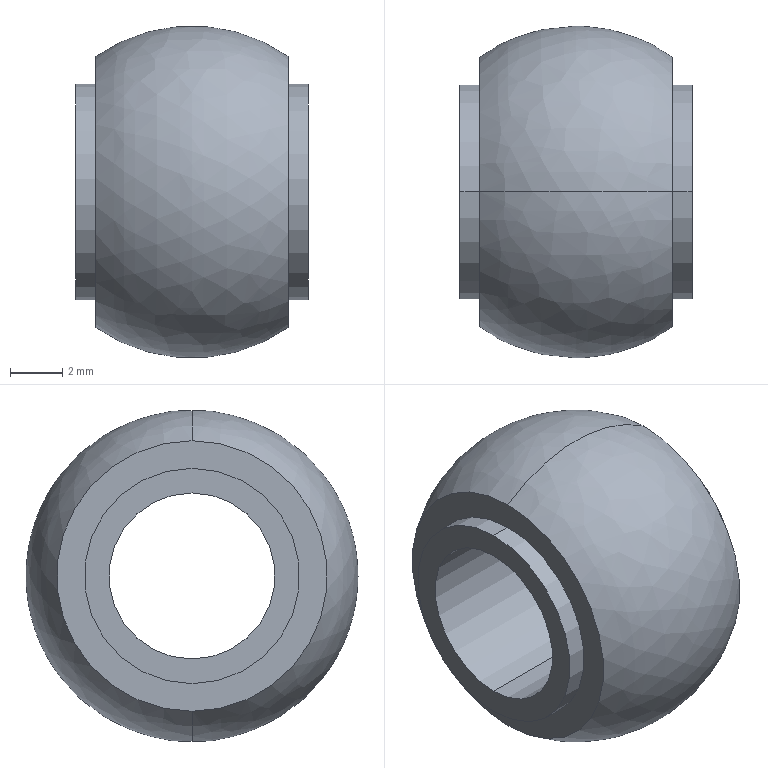Part | SolidWorks | features BaseBody 1 | 1 solid | 12 faces | box 8.89 x 12.647 x 12.7 mm | volume 628.254 mm3 | cylinder 6 | plane 4 | spline 2 | commonest cylinder face diameters 8.243 x4 6.35 x2
STEP:
#1=CARTESIAN_POINT('',(3.683,0.,-5.173));
#2=VERTEX_POINT('',#1);
#3=CARTESIAN_POINT('',(3.683,0.,5.173));
#4=VERTEX_POINT('',#3);
#5=CARTESIAN_POINT('',(3.683,0.,0.));
#6=DIRECTION('',(-1.,0.,0.));
#7=DIRECTION('',(0.,0.,1.));
#8=AXIS2_PLACEMENT_3D('',#5,#6,#7);
#9=CIRCLE('',#8,5.173);
#10=EDGE_CURVE('',#2,#4,#9,.T.);
#11=ORIENTED_EDGE('',*,*,#10,.T.);
#12=CARTESIAN_POINT('',(-3.683,0.,5.173));
#13=VERTEX_POINT('',#12);
#14=CARTESIAN_POINT('',(0.,0.,0.));
#15=DIRECTION('',(0.,-1.,0.));
#16=DIRECTION('',(1.,0.,0.));
#17=AXIS2_PLACEMENT_3D('',#14,#15,#16);
#18=CIRCLE('',#17,6.35);
#19=EDGE_CURVE('',#4,#13,#18,.T.);
#20=ORIENTED_EDGE('',*,*,#19,.T.);
#21=CARTESIAN_POINT('',(-3.683,0.,-5.173));
#22=VERTEX_POINT('',#21);
#23=CARTESIAN_POINT('',(-3.683,0.,0.));
#24=DIRECTION('',(-1.,0.,0.));
#25=DIRECTION('',(0.,0.,1.));
#26=AXIS2_PLACEMENT_3D('',#23,#24,#25);
#27=CIRCLE('',#26,5.173);
#28=EDGE_CURVE('',#22,#13,#27,.T.);
#29=ORIENTED_EDGE('',*,*,#28,.F.);
#30=CARTESIAN_POINT('',(0.,0.,0.));
#31=DIRECTION('',(0.,1.,0.));
#32=DIRECTION('',(1.,0.,0.));
#33=AXIS2_PLACEMENT_3D('',#30,#31,#32);
#34=CIRCLE('',#33,6.35);
#35=EDGE_CURVE('',#2,#22,#34,.T.);
#36=ORIENTED_EDGE('',*,*,#35,.F.);
#37=EDGE_LOOP('',(#11,#20,#29,#36));
#38=FACE_OUTER_BOUND('',#37,.T.);
#39=CARTESIAN_POINT('',(3.683,0.,-5.173));
#40=CARTESIAN_POINT('',(3.683,-10.346,-5.173));
#41=CARTESIAN_POINT('',(3.683,-10.346,5.173));
#42=CARTESIAN_POINT('',(3.683,0.,5.173));
#43=CARTESIAN_POINT('',(1.401,0.,-6.798));
#44=CARTESIAN_POINT('',(1.401,-13.595,-6.798));
#45=CARTESIAN_POINT('',(1.401,-13.595,6.798));
#46=CARTESIAN_POINT('',(1.401,0.,6.798));
#47=CARTESIAN_POINT('',(-1.401,0.,-6.798));
#48=CARTESIAN_POINT('',(-1.401,-13.595,-6.798));
#49=CARTESIAN_POINT('',(-1.401,-13.595,6.798));
#50=CARTESIAN_POINT('',(-1.401,0.,6.798));
#51=CARTESIAN_POINT('',(-3.683,0.,-5.173));
#52=CARTESIAN_POINT('',(-3.683,-10.346,-5.173));
#53=CARTESIAN_POINT('',(-3.683,-10.346,5.173));
#54=CARTESIAN_POINT('',(-3.683,0.,5.173));
#55=(BOUNDED_SURFACE()B_SPLINE_SURFACE(3,3,((#39,#40,#41,#42),(#43,#44,#45,#46),(#47,#48,#49,#50),(#51,#52,#53,#54)),.UNSPECIFIED.,.F.,.F.,.T.)B_SPLINE_SURFACE_WITH_KNOTS((4,4),(4,4),(0.,1.),(0.,1.),.UNSPECIFIED.)GEOMETRIC_REPRESENTATION_ITEM()RATIONAL_B_SPLINE_SURFACE(((1.,0.3333,0.3333,1.),(0.8764,0.2921,0.2921,0.8764),(0.8764,0.2921,0.2921,0.8764),(1.,0.3333,0.3333,1.)))REPRESENTATION_ITEM('')SURFACE());
#56=ADVANCED_FACE('',(#38),#55,.F.);
#57=CARTESIAN_POINT('',(4.445,0.,-4.121));
#58=VERTEX_POINT('',#57);
#59=CARTESIAN_POINT('',(4.445,0.,4.121));
#60=VERTEX_POINT('',#59);
#61=CARTESIAN_POINT('',(4.445,0.,0.));
#62=DIRECTION('',(1.,0.,0.));
#63=DIRECTION('',(0.,0.,1.));
#64=AXIS2_PLACEMENT_3D('',#61,#62,#63);
#65=CIRCLE('',#64,4.121);
#66=EDGE_CURVE('',#58,#60,#65,.T.);
#67=ORIENTED_EDGE('',*,*,#66,.F.);
#68=CARTESIAN_POINT('',(3.683,0.,-4.121));
#69=VERTEX_POINT('',#68);
#70=CARTESIAN_POINT('',(4.445,0.,-4.121));
#71=DIRECTION('',(-1.,0.,0.));
#72=VECTOR('',#71,1000.);
#73=LINE('',#70,#72);
#74=EDGE_CURVE('',#58,#69,#73,.T.);
#75=ORIENTED_EDGE('',*,*,#74,.T.);
#76=CARTESIAN_POINT('',(3.683,0.,4.121));
#77=VERTEX_POINT('',#76);
#78=CARTESIAN_POINT('',(3.683,0.,0.));
#79=DIRECTION('',(-1.,0.,0.));
#80=DIRECTION('',(0.,0.,1.));
#81=AXIS2_PLACEMENT_3D('',#78,#79,#80);
#82=CIRCLE('',#81,4.121);
#83=EDGE_CURVE('',#77,#69,#82,.T.);
#84=ORIENTED_EDGE('',*,*,#83,.F.);
#85=CARTESIAN_POINT('',(4.445,0.,4.121));
#86=DIRECTION('',(-1.,0.,0.));
#87=VECTOR('',#86,1000.);
#88=LINE('',#85,#87);
#89=EDGE_CURVE('',#60,#77,#88,.T.);
#90=ORIENTED_EDGE('',*,*,#89,.F.);
#91=EDGE_LOOP('',(#67,#75,#84,#90));
#92=FACE_OUTER_BOUND('',#91,.T.);
#93=CARTESIAN_POINT('',(4.445,0.,0.));
#94=DIRECTION('',(-1.,0.,0.));
#95=DIRECTION('',(0.,0.,1.));
#96=AXIS2_PLACEMENT_3D('',#93,#94,#95);
#97=CYLINDRICAL_SURFACE('',#96,4.121);
#98=ADVANCED_FACE('',(#92),#97,.T.);
#99=CARTESIAN_POINT('',(4.445,0.,3.175));
#100=VERTEX_POINT('',#99);
#101=CARTESIAN_POINT('',(4.445,0.,-3.175));
#102=VERTEX_POINT('',#101);
#103=CARTESIAN_POINT('',(4.445,0.,0.));
#104=DIRECTION('',(1.,0.,0.));
#105=DIRECTION('',(0.,0.,1.));
#106=AXIS2_PLACEMENT_3D('',#103,#104,#105);
#107=CIRCLE('',#106,3.175);
#108=EDGE_CURVE('',#100,#102,#107,.T.);
#109=ORIENTED_EDGE('',*,*,#108,.T.);
#110=CARTESIAN_POINT('',(-4.445,0.,-3.175));
#111=VERTEX_POINT('',#110);
#112=CARTESIAN_POINT('',(4.445,0.,-3.175));
#113=DIRECTION('',(-1.,0.,0.));
#114=VECTOR('',#113,1000.);
#115=LINE('',#112,#114);
#116=EDGE_CURVE('',#102,#111,#115,.T.);
#117=ORIENTED_EDGE('',*,*,#116,.T.);
#118=CARTESIAN_POINT('',(-4.445,0.,3.175));
#119=VERTEX_POINT('',#118);
#120=CARTESIAN_POINT('',(-4.445,0.,0.));
#121=DIRECTION('',(-1.,0.,0.));
#122=DIRECTION('',(0.,0.,1.));
#123=AXIS2_PLACEMENT_3D('',#120,#121,#122);
#124=CIRCLE('',#123,3.175);
#125=EDGE_CURVE('',#111,#119,#124,.T.);
#126=ORIENTED_EDGE('',*,*,#125,.T.);
#127=CARTESIAN_POINT('',(4.445,0.,3.175));
#128=DIRECTION('',(-1.,0.,0.));
#129=VECTOR('',#128,1000.);
#130=LINE('',#127,#129);
#131=EDGE_CURVE('',#100,#119,#130,.T.);
#132=ORIENTED_EDGE('',*,*,#131,.F.);
#133=EDGE_LOOP('',(#109,#117,#126,#132));
#134=FACE_OUTER_BOUND('',#133,.T.);
#135=CARTESIAN_POINT('',(4.445,0.,0.));
#136=DIRECTION('',(-1.,0.,0.));
#137=DIRECTION('',(0.,0.,1.));
#138=AXIS2_PLACEMENT_3D('',#135,#136,#137);
#139=CYLINDRICAL_SURFACE('',#138,3.175);
#140=ADVANCED_FACE('',(#134),#139,.F.);
#141=CARTESIAN_POINT('',(-3.683,0.,4.121));
#142=VERTEX_POINT('',#141);
#143=CARTESIAN_POINT('',(-3.683,0.,-4.121));
#144=VERTEX_POINT('',#143);
#145=CARTESIAN_POINT('',(-3.683,0.,0.));
#146=DIRECTION('',(-1.,0.,0.));
#147=DIRECTION('',(0.,0.,1.));
#148=AXIS2_PLACEMENT_3D('',#145,#146,#147);
#149=CIRCLE('',#148,4.121);
#150=EDGE_CURVE('',#142,#144,#149,.T.);
#151=ORIENTED_EDGE('',*,*,#150,.T.);
#152=CARTESIAN_POINT('',(-4.445,0.,-4.121));
#153=VERTEX_POINT('',#152);
#154=CARTESIAN_POINT('',(-3.683,0.,-4.121));
#155=DIRECTION('',(-1.,0.,0.));
#156=VECTOR('',#155,1000.);
#157=LINE('',#154,#156);
#158=EDGE_CURVE('',#144,#153,#157,.T.);
#159=ORIENTED_EDGE('',*,*,#158,.T.);
#160=CARTESIAN_POINT('',(-4.445,0.,4.121));
#161=VERTEX_POINT('',#160);
#162=CARTESIAN_POINT('',(-4.445,0.,0.));
#163=DIRECTION('',(1.,0.,0.));
#164=DIRECTION('',(0.,0.,1.));
#165=AXIS2_PLACEMENT_3D('',#162,#163,#164);
#166=CIRCLE('',#165,4.121);
#167=EDGE_CURVE('',#153,#161,#166,.T.);
#168=ORIENTED_EDGE('',*,*,#167,.T.);
#169=CARTESIAN_POINT('',(-3.683,0.,4.121));
#170=DIRECTION('',(-1.,0.,0.));
#171=VECTOR('',#170,1000.);
#172=LINE('',#169,#171);
#173=EDGE_CURVE('',#142,#161,#172,.T.);
#174=ORIENTED_EDGE('',*,*,#173,.F.);
#175=EDGE_LOOP('',(#151,#159,#168,#174));
#176=FACE_OUTER_BOUND('',#175,.T.);
#177=CARTESIAN_POINT('',(-3.683,0.,0.));
#178=DIRECTION('',(-1.,0.,0.));
#179=DIRECTION('',(0.,0.,1.));
#180=AXIS2_PLACEMENT_3D('',#177,#178,#179);
#181=CYLINDRICAL_SURFACE('',#180,4.121);
#182=ADVANCED_FACE('',(#176),#181,.T.);
#183=ORIENTED_EDGE('',*,*,#74,.F.);
#184=CARTESIAN_POINT('',(4.445,0.,0.));
#185=DIRECTION('',(1.,0.,0.));
#186=DIRECTION('',(0.,0.,1.));
#187=AXIS2_PLACEMENT_3D('',#184,#185,#186);
#188=CIRCLE('',#187,4.121);
#189=EDGE_CURVE('',#60,#58,#188,.T.);
#190=ORIENTED_EDGE('',*,*,#189,.F.);
#191=ORIENTED_EDGE('',*,*,#89,.T.);
#192=CARTESIAN_POINT('',(3.683,0.,0.));
#193=DIRECTION('',(-1.,0.,0.));
#194=DIRECTION('',(0.,0.,1.));
#195=AXIS2_PLACEMENT_3D('',#192,#193,#194);
#196=CIRCLE('',#195,4.121);
#197=EDGE_CURVE('',#69,#77,#196,.T.);
#198=ORIENTED_EDGE('',*,*,#197,.F.);
#199=EDGE_LOOP('',(#183,#190,#191,#198));
#200=FACE_OUTER_BOUND('',#199,.T.);
#201=CARTESIAN_POINT('',(4.445,0.,0.));
#202=DIRECTION('',(-1.,0.,0.));
#203=DIRECTION('',(0.,0.,1.));
#204=AXIS2_PLACEMENT_3D('',#201,#202,#203);
#205=CYLINDRICAL_SURFACE('',#204,4.121);
#206=ADVANCED_FACE('',(#200),#205,.T.);
#207=ORIENTED_EDGE('',*,*,#108,.F.);
#208=CARTESIAN_POINT('',(4.445,0.,0.));
#209=DIRECTION('',(1.,0.,0.));
#210=DIRECTION('',(0.,0.,1.));
#211=AXIS2_PLACEMENT_3D('',#208,#209,#210);
#212=CIRCLE('',#211,3.175);
#213=EDGE_CURVE('',#102,#100,#212,.T.);
#214=ORIENTED_EDGE('',*,*,#213,.F.);
#215=EDGE_LOOP('',(#207,#214));
#216=FACE_BOUND('',#215,.T.);
#217=ORIENTED_EDGE('',*,*,#189,.T.);
#218=ORIENTED_EDGE('',*,*,#66,.T.);
#219=EDGE_LOOP('',(#217,#218));
#220=FACE_OUTER_BOUND('',#219,.T.);
#221=CARTESIAN_POINT('',(4.445,-4.171,-4.171));
#222=DIRECTION('',(-1.,0.,0.));
#223=DIRECTION('',(0.,0.,1.));
#224=AXIS2_PLACEMENT_3D('',#221,#222,#223);
#225=PLANE('',#224);
#226=ADVANCED_FACE('',(#216,#220),#225,.F.);
#227=ORIENTED_EDGE('',*,*,#83,.T.);
#228=ORIENTED_EDGE('',*,*,#197,.T.);
#229=EDGE_LOOP('',(#227,#228));
#230=FACE_BOUND('',#229,.T.);
#231=ORIENTED_EDGE('',*,*,#10,.F.);
#232=CARTESIAN_POINT('',(3.683,0.,0.));
#233=DIRECTION('',(-1.,0.,0.));
#234=DIRECTION('',(0.,0.,1.));
#235=AXIS2_PLACEMENT_3D('',#232,#233,#234);
#236=CIRCLE('',#235,5.173);
#237=EDGE_CURVE('',#4,#2,#236,.T.);
#238=ORIENTED_EDGE('',*,*,#237,.F.);
#239=EDGE_LOOP('',(#231,#238));
#240=FACE_OUTER_BOUND('',#239,.T.);
#241=CARTESIAN_POINT('',(3.683,-5.235,-5.235));
#242=DIRECTION('',(-1.,0.,0.));
#243=DIRECTION('',(0.,0.,1.));
#244=AXIS2_PLACEMENT_3D('',#241,#242,#243);
#245=PLANE('',#244);
#246=ADVANCED_FACE('',(#230,#240),#245,.F.);
#247=ORIENTED_EDGE('',*,*,#116,.F.);
#248=ORIENTED_EDGE('',*,*,#213,.T.);
#249=ORIENTED_EDGE('',*,*,#131,.T.);
#250=CARTESIAN_POINT('',(-4.445,0.,0.));
#251=DIRECTION('',(-1.,0.,0.));
#252=DIRECTION('',(0.,0.,1.));
#253=AXIS2_PLACEMENT_3D('',#250,#251,#252);
#254=CIRCLE('',#253,3.175);
#255=EDGE_CURVE('',#119,#111,#254,.T.);
#256=ORIENTED_EDGE('',*,*,#255,.T.);
#257=EDGE_LOOP('',(#247,#248,#249,#256));
#258=FACE_OUTER_BOUND('',#257,.T.);
#259=CARTESIAN_POINT('',(4.445,0.,0.));
#260=DIRECTION('',(-1.,0.,0.));
#261=DIRECTION('',(0.,0.,1.));
#262=AXIS2_PLACEMENT_3D('',#259,#260,#261);
#263=CYLINDRICAL_SURFACE('',#262,3.175);
#264=ADVANCED_FACE('',(#258),#263,.F.);
#265=ORIENTED_EDGE('',*,*,#19,.F.);
#266=ORIENTED_EDGE('',*,*,#237,.T.);
#267=ORIENTED_EDGE('',*,*,#35,.T.);
#268=CARTESIAN_POINT('',(-3.683,0.,0.));
#269=DIRECTION('',(-1.,0.,0.));
#270=DIRECTION('',(0.,0.,1.));
#271=AXIS2_PLACEMENT_3D('',#268,#269,#270);
#272=CIRCLE('',#271,5.173);
#273=EDGE_CURVE('',#13,#22,#272,.T.);
#274=ORIENTED_EDGE('',*,*,#273,.F.);
#275=EDGE_LOOP('',(#265,#266,#267,#274));
#276=FACE_OUTER_BOUND('',#275,.T.);
#277=CARTESIAN_POINT('',(3.683,0.,5.173));
#278=CARTESIAN_POINT('',(3.683,10.346,5.173));
#279=CARTESIAN_POINT('',(3.683,10.346,-5.173));
#280=CARTESIAN_POINT('',(3.683,0.,-5.173));
#281=CARTESIAN_POINT('',(1.401,0.,6.798));
#282=CARTESIAN_POINT('',(1.401,13.595,6.798));
#283=CARTESIAN_POINT('',(1.401,13.595,-6.798));
#284=CARTESIAN_POINT('',(1.401,0.,-6.798));
#285=CARTESIAN_POINT('',(-1.401,0.,6.798));
#286=CARTESIAN_POINT('',(-1.401,13.595,6.798));
#287=CARTESIAN_POINT('',(-1.401,13.595,-6.798));
#288=CARTESIAN_POINT('',(-1.401,0.,-6.798));
#289=CARTESIAN_POINT('',(-3.683,0.,5.173));
#290=CARTESIAN_POINT('',(-3.683,10.346,5.173));
#291=CARTESIAN_POINT('',(-3.683,10.346,-5.173));
#292=CARTESIAN_POINT('',(-3.683,0.,-5.173));
#293=(BOUNDED_SURFACE()B_SPLINE_SURFACE(3,3,((#277,#278,#279,#280),(#281,#282,#283,#284),(#285,#286,#287,#288),(#289,#290,#291,#292)),.UNSPECIFIED.,.F.,.F.,.F.)B_SPLINE_SURFACE_WITH_KNOTS((4,4),(4,4),(0.,1.),(0.,1.),.UNSPECIFIED.)GEOMETRIC_REPRESENTATION_ITEM()RATIONAL_B_SPLINE_SURFACE(((1.,0.3333,0.3333,1.),(0.8764,0.2921,0.2921,0.8764),(0.8764,0.2921,0.2921,0.8764),(1.,0.3333,0.3333,1.)))REPRESENTATION_ITEM('')SURFACE());
#294=ADVANCED_FACE('',(#276),#293,.F.);
#295=ORIENTED_EDGE('',*,*,#255,.F.);
#296=ORIENTED_EDGE('',*,*,#125,.F.);
#297=EDGE_LOOP('',(#295,#296));
#298=FACE_BOUND('',#297,.T.);
#299=CARTESIAN_POINT('',(-4.445,0.,0.));
#300=DIRECTION('',(1.,0.,0.));
#301=DIRECTION('',(0.,0.,1.));
#302=AXIS2_PLACEMENT_3D('',#299,#300,#301);
#303=CIRCLE('',#302,4.121);
#304=EDGE_CURVE('',#161,#153,#303,.T.);
#305=ORIENTED_EDGE('',*,*,#304,.F.);
#306=ORIENTED_EDGE('',*,*,#167,.F.);
#307=EDGE_LOOP('',(#305,#306));
#308=FACE_OUTER_BOUND('',#307,.T.);
#309=CARTESIAN_POINT('',(-4.445,-4.171,4.171));
#310=DIRECTION('',(1.,0.,0.));
#311=DIRECTION('',(0.,0.,-1.));
#312=AXIS2_PLACEMENT_3D('',#309,#310,#311);
#313=PLANE('',#312);
#314=ADVANCED_FACE('',(#298,#308),#313,.F.);
#315=ORIENTED_EDGE('',*,*,#150,.F.);
#316=CARTESIAN_POINT('',(-3.683,0.,0.));
#317=DIRECTION('',(-1.,0.,0.));
#318=DIRECTION('',(0.,0.,1.));
#319=AXIS2_PLACEMENT_3D('',#316,#317,#318);
#320=CIRCLE('',#319,4.121);
#321=EDGE_CURVE('',#144,#142,#320,.T.);
#322=ORIENTED_EDGE('',*,*,#321,.F.);
#323=EDGE_LOOP('',(#315,#322));
#324=FACE_BOUND('',#323,.T.);
#325=ORIENTED_EDGE('',*,*,#28,.T.);
#326=ORIENTED_EDGE('',*,*,#273,.T.);
#327=EDGE_LOOP('',(#325,#326));
#328=FACE_OUTER_BOUND('',#327,.T.);
#329=CARTESIAN_POINT('',(-3.683,-5.235,5.235));
#330=DIRECTION('',(1.,0.,0.));
#331=DIRECTION('',(0.,0.,-1.));
#332=AXIS2_PLACEMENT_3D('',#329,#330,#331);
#333=PLANE('',#332);
#334=ADVANCED_FACE('',(#324,#328),#333,.F.);
#335=ORIENTED_EDGE('',*,*,#158,.F.);
#336=ORIENTED_EDGE('',*,*,#321,.T.);
#337=ORIENTED_EDGE('',*,*,#173,.T.);
#338=ORIENTED_EDGE('',*,*,#304,.T.);
#339=EDGE_LOOP('',(#335,#336,#337,#338));
#340=FACE_OUTER_BOUND('',#339,.T.);
#341=CARTESIAN_POINT('',(-3.683,0.,0.));
#342=DIRECTION('',(-1.,0.,0.));
#343=DIRECTION('',(0.,0.,1.));
#344=AXIS2_PLACEMENT_3D('',#341,#342,#343);
#345=CYLINDRICAL_SURFACE('',#344,4.121);
#346=ADVANCED_FACE('',(#340),#345,.T.);
#347=CLOSED_SHELL('',(#56,#98,#140,#182,#206,#226,#246,#264,#294,#314,#334,#346));
#348=MANIFOLD_SOLID_BREP('',#347);
#349=CARTESIAN_POINT('',(0.,0.,0.));
#350=DIRECTION('',(0.,0.,1.));
#351=DIRECTION('',(1.,0.,0.));
#352=AXIS2_PLACEMENT_3D('',#349,#350,#351);
#353=(LENGTH_UNIT()NAMED_UNIT(*)SI_UNIT(.MILLI.,.METRE.));
#354=UNCERTAINTY_MEASURE_WITH_UNIT(LENGTH_MEASURE(0.00001),#353,'','');
#355=(NAMED_UNIT(*)PLANE_ANGLE_UNIT()SI_UNIT($,.RADIAN.));
#356=(NAMED_UNIT(*)SI_UNIT($,.STERADIAN.)SOLID_ANGLE_UNIT());
#357=(GEOMETRIC_REPRESENTATION_CONTEXT(3)GLOBAL_UNCERTAINTY_ASSIGNED_CONTEXT((#354))GLOBAL_UNIT_ASSIGNED_CONTEXT((#353,#355,#356))REPRESENTATION_CONTEXT('',''));
#358=ADVANCED_BREP_SHAPE_REPRESENTATION('',(#348,#352),#357);